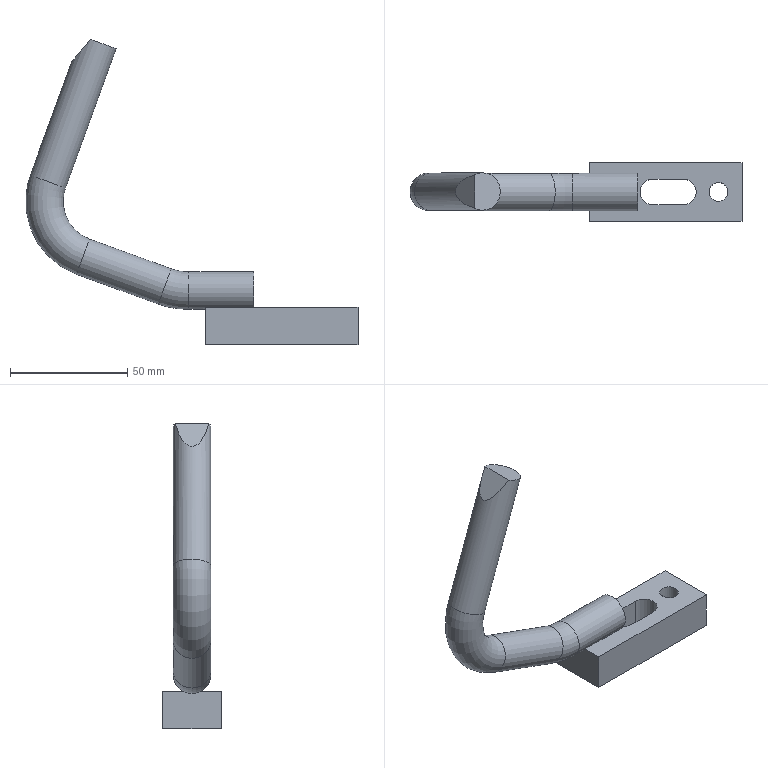Part | NX | features MAIN_BODY 2 | 1 solid | 19 faces | box 141.738 x 25 x 130.205 mm | volume 56808 mm3 | plane 10 | cylinder 6 | torus 2 | spline 1 | commonest cylinder face diameters 16 x3 11 x2 8 x1
STEP:
#1=CARTESIAN_POINT('',(970.,301.373,-139.));
#2=VERTEX_POINT('',#1);
#3=CARTESIAN_POINT('',(970.,293.627,-139.));
#4=VERTEX_POINT('',#3);
#5=CARTESIAN_POINT('',(970.,297.5,-132.));
#6=DIRECTION('',(1.,0.,0.));
#7=DIRECTION('',(0.,1.,0.));
#8=AXIS2_PLACEMENT_3D('',#5,#6,#7);
#9=CIRCLE('',#8,8.);
#10=EDGE_CURVE('',#2,#4,#9,.F.);
#11=ORIENTED_EDGE('',*,*,#10,.F.);
#12=CARTESIAN_POINT('',(970.,310.,-139.));
#13=VERTEX_POINT('',#12);
#14=CARTESIAN_POINT('',(970.,285.5,-139.));
#15=DIRECTION('',(0.,-1.,0.));
#16=VECTOR('',#15,1000.);
#17=LINE('',#14,#16);
#18=EDGE_CURVE('',#2,#13,#17,.F.);
#19=ORIENTED_EDGE('',*,*,#18,.T.);
#20=CARTESIAN_POINT('',(970.,310.,-155.));
#21=VERTEX_POINT('',#20);
#22=CARTESIAN_POINT('',(970.,310.,-135.));
#23=DIRECTION('',(0.,0.,1.));
#24=VECTOR('',#23,1000.);
#25=LINE('',#22,#24);
#26=EDGE_CURVE('',#21,#13,#25,.T.);
#27=ORIENTED_EDGE('',*,*,#26,.F.);
#28=CARTESIAN_POINT('',(970.,285.,-155.));
#29=VERTEX_POINT('',#28);
#30=CARTESIAN_POINT('',(970.,285.5,-155.));
#31=DIRECTION('',(0.,-1.,0.));
#32=VECTOR('',#31,1000.);
#33=LINE('',#30,#32);
#34=EDGE_CURVE('',#29,#21,#33,.F.);
#35=ORIENTED_EDGE('',*,*,#34,.F.);
#36=CARTESIAN_POINT('',(970.,285.,-139.));
#37=VERTEX_POINT('',#36);
#38=CARTESIAN_POINT('',(970.,285.,-135.));
#39=DIRECTION('',(0.,0.,-1.));
#40=VECTOR('',#39,1000.);
#41=LINE('',#38,#40);
#42=EDGE_CURVE('',#29,#37,#41,.F.);
#43=ORIENTED_EDGE('',*,*,#42,.T.);
#44=CARTESIAN_POINT('',(970.,285.5,-139.));
#45=DIRECTION('',(0.,-1.,0.));
#46=VECTOR('',#45,1000.);
#47=LINE('',#44,#46);
#48=EDGE_CURVE('',#37,#4,#47,.F.);
#49=ORIENTED_EDGE('',*,*,#48,.T.);
#50=EDGE_LOOP('',(#11,#19,#27,#35,#43,#49));
#51=FACE_BOUND('',#50,.T.);
#52=CARTESIAN_POINT('',(970.,285.5,-135.));
#53=DIRECTION('',(1.,0.,0.));
#54=DIRECTION('',(0.,1.,0.));
#55=AXIS2_PLACEMENT_3D('',#52,#53,#54);
#56=PLANE('',#55);
#57=ADVANCED_FACE('',(#51),#56,.F.);
#58=ORIENTED_EDGE('',*,*,#18,.F.);
#59=CARTESIAN_POINT('',(990.552,301.373,-139.));
#60=VERTEX_POINT('',#59);
#61=CARTESIAN_POINT('',(962.842,301.373,-139.));
#62=DIRECTION('',(1.,0.,0.));
#63=VECTOR('',#62,1000.);
#64=LINE('',#61,#63);
#65=EDGE_CURVE('',#2,#60,#64,.T.);
#66=ORIENTED_EDGE('',*,*,#65,.T.);
#67=CARTESIAN_POINT('',(990.552,293.627,-139.));
#68=VERTEX_POINT('',#67);
#69=CARTESIAN_POINT('',(990.552,285.5,-139.));
#70=DIRECTION('',(0.,-1.,0.));
#71=VECTOR('',#70,1000.);
#72=LINE('',#69,#71);
#73=EDGE_CURVE('',#60,#68,#72,.T.);
#74=ORIENTED_EDGE('',*,*,#73,.T.);
#75=CARTESIAN_POINT('',(962.842,293.627,-139.));
#76=DIRECTION('',(1.,0.,0.));
#77=VECTOR('',#76,1000.);
#78=LINE('',#75,#77);
#79=EDGE_CURVE('',#68,#4,#78,.F.);
#80=ORIENTED_EDGE('',*,*,#79,.T.);
#81=ORIENTED_EDGE('',*,*,#48,.F.);
#82=CARTESIAN_POINT('',(1035.,285.,-139.));
#83=VERTEX_POINT('',#82);
#84=CARTESIAN_POINT('',(900.,285.,-139.));
#85=DIRECTION('',(1.,0.,0.));
#86=VECTOR('',#85,1000.);
#87=LINE('',#84,#86);
#88=EDGE_CURVE('',#37,#83,#87,.T.);
#89=ORIENTED_EDGE('',*,*,#88,.T.);
#90=CARTESIAN_POINT('',(1035.,310.,-139.));
#91=VERTEX_POINT('',#90);
#92=CARTESIAN_POINT('',(1035.,285.5,-139.));
#93=DIRECTION('',(0.,1.,0.));
#94=VECTOR('',#93,1000.);
#95=LINE('',#92,#94);
#96=EDGE_CURVE('',#83,#91,#95,.T.);
#97=ORIENTED_EDGE('',*,*,#96,.T.);
#98=CARTESIAN_POINT('',(900.,310.,-139.));
#99=DIRECTION('',(-1.,0.,0.));
#100=VECTOR('',#99,1000.);
#101=LINE('',#98,#100);
#102=EDGE_CURVE('',#13,#91,#101,.F.);
#103=ORIENTED_EDGE('',*,*,#102,.F.);
#104=EDGE_LOOP('',(#58,#66,#74,#80,#81,#89,#97,#103));
#105=FACE_BOUND('',#104,.T.);
#106=CARTESIAN_POINT('',(1021.,297.5,-139.));
#107=VERTEX_POINT('',#106);
#108=CARTESIAN_POINT('',(1025.,297.5,-139.));
#109=DIRECTION('',(0.,0.,-1.));
#110=DIRECTION('',(-1.,0.,0.));
#111=AXIS2_PLACEMENT_3D('',#108,#109,#110);
#112=CIRCLE('',#111,4.);
#113=EDGE_CURVE('',#107,#107,#112,.F.);
#114=ORIENTED_EDGE('',*,*,#113,.F.);
#115=EDGE_LOOP('',(#114));
#116=FACE_BOUND('',#115,.T.);
#117=CARTESIAN_POINT('',(1010.,292.,-139.));
#118=VERTEX_POINT('',#117);
#119=CARTESIAN_POINT('',(1010.,303.,-139.));
#120=VERTEX_POINT('',#119);
#121=CARTESIAN_POINT('',(1010.,297.5,-139.));
#122=DIRECTION('',(0.,0.,-1.));
#123=DIRECTION('',(-1.,0.,0.));
#124=AXIS2_PLACEMENT_3D('',#121,#122,#123);
#125=CIRCLE('',#124,5.5);
#126=EDGE_CURVE('',#118,#120,#125,.F.);
#127=ORIENTED_EDGE('',*,*,#126,.F.);
#128=CARTESIAN_POINT('',(997.,292.,-139.));
#129=VERTEX_POINT('',#128);
#130=CARTESIAN_POINT('',(969.,292.,-139.));
#131=DIRECTION('',(-1.,0.,0.));
#132=VECTOR('',#131,1000.);
#133=LINE('',#130,#132);
#134=EDGE_CURVE('',#129,#118,#133,.F.);
#135=ORIENTED_EDGE('',*,*,#134,.F.);
#136=CARTESIAN_POINT('',(997.,303.,-139.));
#137=VERTEX_POINT('',#136);
#138=CARTESIAN_POINT('',(997.,297.5,-139.));
#139=DIRECTION('',(0.,0.,-1.));
#140=DIRECTION('',(-1.,0.,0.));
#141=AXIS2_PLACEMENT_3D('',#138,#139,#140);
#142=CIRCLE('',#141,5.5);
#143=EDGE_CURVE('',#137,#129,#142,.F.);
#144=ORIENTED_EDGE('',*,*,#143,.F.);
#145=CARTESIAN_POINT('',(969.,303.,-139.));
#146=DIRECTION('',(-1.,0.,0.));
#147=VECTOR('',#146,1000.);
#148=LINE('',#145,#147);
#149=EDGE_CURVE('',#120,#137,#148,.T.);
#150=ORIENTED_EDGE('',*,*,#149,.F.);
#151=EDGE_LOOP('',(#127,#135,#144,#150));
#152=FACE_BOUND('',#151,.T.);
#153=CARTESIAN_POINT('',(900.,285.5,-139.));
#154=DIRECTION('',(0.,0.,-1.));
#155=DIRECTION('',(-1.,0.,0.));
#156=AXIS2_PLACEMENT_3D('',#153,#154,#155);
#157=PLANE('',#156);
#158=ADVANCED_FACE('',(#105,#116,#152),#157,.F.);
#159=CARTESIAN_POINT('',(1035.,285.,-155.));
#160=VERTEX_POINT('',#159);
#161=CARTESIAN_POINT('',(1035.,285.,-135.));
#162=DIRECTION('',(0.,0.,1.));
#163=VECTOR('',#162,1000.);
#164=LINE('',#161,#163);
#165=EDGE_CURVE('',#160,#83,#164,.T.);
#166=ORIENTED_EDGE('',*,*,#165,.T.);
#167=ORIENTED_EDGE('',*,*,#88,.F.);
#168=ORIENTED_EDGE('',*,*,#42,.F.);
#169=CARTESIAN_POINT('',(900.,285.,-155.));
#170=DIRECTION('',(1.,0.,0.));
#171=VECTOR('',#170,1000.);
#172=LINE('',#169,#171);
#173=EDGE_CURVE('',#29,#160,#172,.T.);
#174=ORIENTED_EDGE('',*,*,#173,.T.);
#175=EDGE_LOOP('',(#166,#167,#168,#174));
#176=FACE_BOUND('',#175,.T.);
#177=CARTESIAN_POINT('',(900.,285.,-135.));
#178=DIRECTION('',(0.,-1.,0.));
#179=DIRECTION('',(1.,0.,0.));
#180=AXIS2_PLACEMENT_3D('',#177,#178,#179);
#181=PLANE('',#180);
#182=ADVANCED_FACE('',(#176),#181,.T.);
#183=ORIENTED_EDGE('',*,*,#26,.T.);
#184=ORIENTED_EDGE('',*,*,#102,.T.);
#185=CARTESIAN_POINT('',(1035.,310.,-155.));
#186=VERTEX_POINT('',#185);
#187=CARTESIAN_POINT('',(1035.,310.,-135.));
#188=DIRECTION('',(0.,0.,-1.));
#189=VECTOR('',#188,1000.);
#190=LINE('',#187,#189);
#191=EDGE_CURVE('',#186,#91,#190,.F.);
#192=ORIENTED_EDGE('',*,*,#191,.F.);
#193=CARTESIAN_POINT('',(900.,310.,-155.));
#194=DIRECTION('',(-1.,0.,0.));
#195=VECTOR('',#194,1000.);
#196=LINE('',#193,#195);
#197=EDGE_CURVE('',#21,#186,#196,.F.);
#198=ORIENTED_EDGE('',*,*,#197,.F.);
#199=EDGE_LOOP('',(#183,#184,#192,#198));
#200=FACE_BOUND('',#199,.T.);
#201=CARTESIAN_POINT('',(900.,310.,-135.));
#202=DIRECTION('',(0.,-1.,0.));
#203=DIRECTION('',(1.,0.,0.));
#204=AXIS2_PLACEMENT_3D('',#201,#202,#203);
#205=PLANE('',#204);
#206=ADVANCED_FACE('',(#200),#205,.F.);
#207=CARTESIAN_POINT('',(1035.,285.5,-155.));
#208=DIRECTION('',(0.,1.,0.));
#209=VECTOR('',#208,1000.);
#210=LINE('',#207,#209);
#211=EDGE_CURVE('',#160,#186,#210,.T.);
#212=ORIENTED_EDGE('',*,*,#211,.T.);
#213=ORIENTED_EDGE('',*,*,#191,.T.);
#214=ORIENTED_EDGE('',*,*,#96,.F.);
#215=ORIENTED_EDGE('',*,*,#165,.F.);
#216=EDGE_LOOP('',(#212,#213,#214,#215));
#217=FACE_BOUND('',#216,.T.);
#218=CARTESIAN_POINT('',(1035.,285.5,-135.));
#219=DIRECTION('',(1.,0.,0.));
#220=DIRECTION('',(0.,1.,0.));
#221=AXIS2_PLACEMENT_3D('',#218,#219,#220);
#222=PLANE('',#221);
#223=ADVANCED_FACE('',(#217),#222,.T.);
#224=CARTESIAN_POINT('',(1021.03,297.987,-155.));
#225=VERTEX_POINT('',#224);
#226=CARTESIAN_POINT('',(1025.,297.5,-155.));
#227=DIRECTION('',(0.,0.,1.));
#228=DIRECTION('',(-0.9925,0.1219,0.));
#229=AXIS2_PLACEMENT_3D('',#226,#227,#228);
#230=CIRCLE('',#229,4.);
#231=EDGE_CURVE('',#225,#225,#230,.T.);
#232=ORIENTED_EDGE('',*,*,#231,.T.);
#233=EDGE_LOOP('',(#232));
#234=FACE_BOUND('',#233,.T.);
#235=CARTESIAN_POINT('',(1010.,303.,-155.));
#236=VERTEX_POINT('',#235);
#237=CARTESIAN_POINT('',(997.,303.,-155.));
#238=VERTEX_POINT('',#237);
#239=CARTESIAN_POINT('',(969.,303.,-155.));
#240=DIRECTION('',(-1.,0.,0.));
#241=VECTOR('',#240,1000.);
#242=LINE('',#239,#241);
#243=EDGE_CURVE('',#236,#238,#242,.T.);
#244=ORIENTED_EDGE('',*,*,#243,.T.);
#245=CARTESIAN_POINT('',(997.,292.,-155.));
#246=VERTEX_POINT('',#245);
#247=CARTESIAN_POINT('',(997.,297.5,-155.));
#248=DIRECTION('',(0.,0.,-1.));
#249=DIRECTION('',(-0.9925,0.1219,0.));
#250=AXIS2_PLACEMENT_3D('',#247,#248,#249);
#251=CIRCLE('',#250,5.5);
#252=EDGE_CURVE('',#238,#246,#251,.F.);
#253=ORIENTED_EDGE('',*,*,#252,.T.);
#254=CARTESIAN_POINT('',(1010.,292.,-155.));
#255=VERTEX_POINT('',#254);
#256=CARTESIAN_POINT('',(969.,292.,-155.));
#257=DIRECTION('',(-1.,0.,0.));
#258=VECTOR('',#257,1000.);
#259=LINE('',#256,#258);
#260=EDGE_CURVE('',#246,#255,#259,.F.);
#261=ORIENTED_EDGE('',*,*,#260,.T.);
#262=CARTESIAN_POINT('',(1010.,297.5,-155.));
#263=DIRECTION('',(0.,0.,-1.));
#264=DIRECTION('',(-0.9925,0.1219,0.));
#265=AXIS2_PLACEMENT_3D('',#262,#263,#264);
#266=CIRCLE('',#265,5.5);
#267=EDGE_CURVE('',#255,#236,#266,.F.);
#268=ORIENTED_EDGE('',*,*,#267,.T.);
#269=EDGE_LOOP('',(#244,#253,#261,#268));
#270=FACE_BOUND('',#269,.T.);
#271=ORIENTED_EDGE('',*,*,#197,.T.);
#272=ORIENTED_EDGE('',*,*,#211,.F.);
#273=ORIENTED_EDGE('',*,*,#173,.F.);
#274=ORIENTED_EDGE('',*,*,#34,.T.);
#275=EDGE_LOOP('',(#271,#272,#273,#274));
#276=FACE_BOUND('',#275,.T.);
#277=CARTESIAN_POINT('',(900.,285.5,-155.));
#278=DIRECTION('',(0.,0.,-1.));
#279=DIRECTION('',(-1.,0.,0.));
#280=AXIS2_PLACEMENT_3D('',#277,#278,#279);
#281=PLANE('',#280);
#282=ADVANCED_FACE('',(#234,#270,#276),#281,.T.);
#283=ORIENTED_EDGE('',*,*,#143,.T.);
#284=CARTESIAN_POINT('',(997.,292.,-119.));
#285=DIRECTION('',(0.,0.,-1.));
#286=VECTOR('',#285,1000.);
#287=LINE('',#284,#286);
#288=EDGE_CURVE('',#129,#246,#287,.T.);
#289=ORIENTED_EDGE('',*,*,#288,.T.);
#290=ORIENTED_EDGE('',*,*,#252,.F.);
#291=CARTESIAN_POINT('',(997.,303.,-119.));
#292=DIRECTION('',(0.,0.,-1.));
#293=VECTOR('',#292,1000.);
#294=LINE('',#291,#293);
#295=EDGE_CURVE('',#137,#238,#294,.T.);
#296=ORIENTED_EDGE('',*,*,#295,.F.);
#297=EDGE_LOOP('',(#283,#289,#290,#296));
#298=FACE_BOUND('',#297,.T.);
#299=CARTESIAN_POINT('',(997.,297.5,-119.));
#300=DIRECTION('',(0.,0.,-1.));
#301=DIRECTION('',(-1.,0.,0.));
#302=AXIS2_PLACEMENT_3D('',#299,#300,#301);
#303=CYLINDRICAL_SURFACE('',#302,5.5);
#304=ADVANCED_FACE('',(#298),#303,.F.);
#305=ORIENTED_EDGE('',*,*,#126,.T.);
#306=CARTESIAN_POINT('',(1010.,303.,-119.));
#307=DIRECTION('',(0.,0.,-1.));
#308=VECTOR('',#307,1000.);
#309=LINE('',#306,#308);
#310=EDGE_CURVE('',#120,#236,#309,.T.);
#311=ORIENTED_EDGE('',*,*,#310,.T.);
#312=ORIENTED_EDGE('',*,*,#267,.F.);
#313=CARTESIAN_POINT('',(1010.,292.,-119.));
#314=DIRECTION('',(0.,0.,-1.));
#315=VECTOR('',#314,1000.);
#316=LINE('',#313,#315);
#317=EDGE_CURVE('',#118,#255,#316,.T.);
#318=ORIENTED_EDGE('',*,*,#317,.F.);
#319=EDGE_LOOP('',(#305,#311,#312,#318));
#320=FACE_BOUND('',#319,.T.);
#321=CARTESIAN_POINT('',(1010.,297.5,-119.));
#322=DIRECTION('',(0.,0.,-1.));
#323=DIRECTION('',(-1.,0.,0.));
#324=AXIS2_PLACEMENT_3D('',#321,#322,#323);
#325=CYLINDRICAL_SURFACE('',#324,5.5);
#326=ADVANCED_FACE('',(#320),#325,.F.);
#327=ORIENTED_EDGE('',*,*,#310,.F.);
#328=ORIENTED_EDGE('',*,*,#149,.T.);
#329=ORIENTED_EDGE('',*,*,#295,.T.);
#330=ORIENTED_EDGE('',*,*,#243,.F.);
#331=EDGE_LOOP('',(#327,#328,#329,#330));
#332=FACE_BOUND('',#331,.T.);
#333=CARTESIAN_POINT('',(969.,303.,-119.));
#334=DIRECTION('',(0.,1.,0.));
#335=DIRECTION('',(-1.,0.,0.));
#336=AXIS2_PLACEMENT_3D('',#333,#334,#335);
#337=PLANE('',#336);
#338=ADVANCED_FACE('',(#332),#337,.F.);
#339=ORIENTED_EDGE('',*,*,#288,.F.);
#340=ORIENTED_EDGE('',*,*,#134,.T.);
#341=ORIENTED_EDGE('',*,*,#317,.T.);
#342=ORIENTED_EDGE('',*,*,#260,.F.);
#343=EDGE_LOOP('',(#339,#340,#341,#342));
#344=FACE_BOUND('',#343,.T.);
#345=CARTESIAN_POINT('',(969.,292.,-119.));
#346=DIRECTION('',(0.,1.,0.));
#347=DIRECTION('',(-1.,0.,0.));
#348=AXIS2_PLACEMENT_3D('',#345,#346,#347);
#349=PLANE('',#348);
#350=ADVANCED_FACE('',(#344),#349,.T.);
#351=ORIENTED_EDGE('',*,*,#231,.F.);
#352=EDGE_LOOP('',(#351));
#353=FACE_BOUND('',#352,.T.);
#354=ORIENTED_EDGE('',*,*,#113,.T.);
#355=EDGE_LOOP('',(#354));
#356=FACE_BOUND('',#355,.T.);
#357=CARTESIAN_POINT('',(1025.,297.5,-139.));
#358=DIRECTION('',(0.,0.,-1.));
#359=DIRECTION('',(-0.9925,0.1219,0.));
#360=AXIS2_PLACEMENT_3D('',#357,#358,#359);
#361=CYLINDRICAL_SURFACE('',#360,4.);
#362=ADVANCED_FACE('',(#353,#356),#361,.F.);
#363=CARTESIAN_POINT('',(962.842,297.5,-140.));
#364=VERTEX_POINT('',#363);
#365=CARTESIAN_POINT('',(962.842,297.5,-132.));
#366=DIRECTION('',(1.,0.,0.));
#367=DIRECTION('',(0.,0.,-1.));
#368=AXIS2_PLACEMENT_3D('',#365,#366,#367);
#369=CIRCLE('',#368,8.);
#370=EDGE_CURVE('',#364,#364,#369,.T.);
#371=ORIENTED_EDGE('',*,*,#370,.T.);
#372=EDGE_LOOP('',(#371));
#373=FACE_BOUND('',#372,.T.);
#374=ORIENTED_EDGE('',*,*,#65,.F.);
#375=ORIENTED_EDGE('',*,*,#10,.T.);
#376=ORIENTED_EDGE('',*,*,#79,.F.);
#377=CARTESIAN_POINT('',(990.552,297.5,-132.));
#378=DIRECTION('',(1.,0.,0.));
#379=DIRECTION('',(0.,0.,-1.));
#380=AXIS2_PLACEMENT_3D('',#377,#378,#379);
#381=CIRCLE('',#380,8.);
#382=EDGE_CURVE('',#60,#68,#381,.T.);
#383=ORIENTED_EDGE('',*,*,#382,.F.);
#384=EDGE_LOOP('',(#374,#375,#376,#383));
#385=FACE_BOUND('',#384,.T.);
#386=CARTESIAN_POINT('',(962.842,297.5,-132.));
#387=DIRECTION('',(1.,0.,0.));
#388=DIRECTION('',(0.,0.,-1.));
#389=AXIS2_PLACEMENT_3D('',#386,#387,#388);
#390=CYLINDRICAL_SURFACE('',#389,8.);
#391=ADVANCED_FACE('',(#373,#385),#390,.T.);
#392=ORIENTED_EDGE('',*,*,#73,.F.);
#393=ORIENTED_EDGE('',*,*,#382,.T.);
#394=EDGE_LOOP('',(#392,#393));
#395=FACE_BOUND('',#394,.T.);
#396=CARTESIAN_POINT('',(990.552,297.5,-132.));
#397=DIRECTION('',(1.,0.,0.));
#398=DIRECTION('',(0.,0.,-1.));
#399=AXIS2_PLACEMENT_3D('',#396,#397,#398);
#400=PLANE('',#399);
#401=ADVANCED_FACE('',(#395),#400,.T.);
#402=CARTESIAN_POINT('',(895.252,297.5,-82.72));
#403=VERTEX_POINT('',#402);
#404=CARTESIAN_POINT('',(902.769,297.5,-85.456));
#405=DIRECTION('',(-0.342,0.,-0.9397));
#406=DIRECTION('',(-0.9397,0.,0.342));
#407=AXIS2_PLACEMENT_3D('',#404,#405,#406);
#408=CIRCLE('',#407,8.);
#409=EDGE_CURVE('',#403,#403,#408,.T.);
#410=ORIENTED_EDGE('',*,*,#409,.F.);
#411=EDGE_LOOP('',(#410));
#412=FACE_BOUND('',#411,.T.);
#413=CARTESIAN_POINT('',(920.975,304.624,-24.795));
#414=VERTEX_POINT('',#413);
#415=CARTESIAN_POINT('',(920.975,290.376,-24.795));
#416=VERTEX_POINT('',#415);
#417=CARTESIAN_POINT('',(924.395,297.5,-26.04));
#418=DIRECTION('',(-0.342,0.,-0.9397));
#419=DIRECTION('',(-0.9397,0.,0.342));
#420=AXIS2_PLACEMENT_3D('',#417,#418,#419);
#421=CIRCLE('',#420,8.);
#422=EDGE_CURVE('',#414,#416,#421,.T.);
#423=ORIENTED_EDGE('',*,*,#422,.T.);
#424=CARTESIAN_POINT('',(920.975,290.376,-24.795));
#425=CARTESIAN_POINT('',(920.16,290.597,-25.766));
#426=CARTESIAN_POINT('',(918.549,291.134,-27.686));
#427=CARTESIAN_POINT('',(916.586,292.114,-30.026));
#428=CARTESIAN_POINT('',(915.08,293.202,-31.821));
#429=CARTESIAN_POINT('',(914.033,294.226,-33.068));
#430=CARTESIAN_POINT('',(913.117,295.557,-34.16));
#431=CARTESIAN_POINT('',(912.618,297.47,-34.754));
#432=CARTESIAN_POINT('',(913.094,299.401,-34.187));
#433=CARTESIAN_POINT('',(914.014,300.754,-33.091));
#434=CARTESIAN_POINT('',(915.069,301.79,-31.834));
#435=CARTESIAN_POINT('',(916.584,302.886,-30.027));
#436=CARTESIAN_POINT('',(918.541,303.862,-27.696));
#437=CARTESIAN_POINT('',(920.158,304.402,-25.769));
#438=CARTESIAN_POINT('',(920.975,304.624,-24.795));
#439=B_SPLINE_CURVE_WITH_KNOTS('',3,(#424,#425,#426,#427,#428,#429,#430,#431,#432,#433,#434,#435,#436,#437,#438),.UNSPECIFIED.,.F.,.F.,(4,1,1,1,1,1,1,1,1,1,1,1,4),(0.,0.00384,0.00768,0.0096,0.01152,0.01344,0.01536,0.01728,0.0192,0.02112,0.02304,0.02688,0.03072),.UNSPECIFIED.);
#440=EDGE_CURVE('',#416,#414,#439,.T.);
#441=ORIENTED_EDGE('',*,*,#440,.T.);
#442=EDGE_LOOP('',(#423,#441));
#443=FACE_BOUND('',#442,.T.);
#444=CARTESIAN_POINT('',(902.769,297.5,-85.456));
#445=DIRECTION('',(0.342,0.,0.9397));
#446=DIRECTION('',(0.9397,0.,-0.342));
#447=AXIS2_PLACEMENT_3D('',#444,#445,#446);
#448=CYLINDRICAL_SURFACE('',#447,8.);
#449=ADVANCED_FACE('',(#412,#443),#448,.T.);
#450=CARTESIAN_POINT('',(914.975,297.5,-125.017));
#451=VERTEX_POINT('',#450);
#452=CARTESIAN_POINT('',(917.711,297.5,-117.499));
#453=DIRECTION('',(0.9397,0.,-0.342));
#454=DIRECTION('',(-0.342,0.,-0.9397));
#455=AXIS2_PLACEMENT_3D('',#452,#453,#454);
#456=CIRCLE('',#455,8.);
#457=EDGE_CURVE('',#451,#451,#456,.T.);
#458=ORIENTED_EDGE('',*,*,#457,.F.);
#459=EDGE_LOOP('',(#458));
#460=FACE_BOUND('',#459,.T.);
#461=ORIENTED_EDGE('',*,*,#409,.T.);
#462=EDGE_LOOP('',(#461));
#463=FACE_BOUND('',#462,.T.);
#464=CARTESIAN_POINT('',(926.262,297.5,-94.007));
#465=DIRECTION('',(0.,1.,0.));
#466=DIRECTION('',(0.,0.,1.));
#467=AXIS2_PLACEMENT_3D('',#464,#465,#466);
#468=TOROIDAL_SURFACE('',#467,25.,8.);
#469=ADVANCED_FACE('',(#460,#463),#468,.T.);
#470=CARTESIAN_POINT('',(949.845,297.5,-137.708));
#471=VERTEX_POINT('',#470);
#472=CARTESIAN_POINT('',(952.581,297.5,-130.191));
#473=DIRECTION('',(0.9397,0.,-0.342));
#474=DIRECTION('',(-0.342,0.,-0.9397));
#475=AXIS2_PLACEMENT_3D('',#472,#473,#474);
#476=CIRCLE('',#475,8.);
#477=EDGE_CURVE('',#471,#471,#476,.T.);
#478=ORIENTED_EDGE('',*,*,#477,.F.);
#479=EDGE_LOOP('',(#478));
#480=FACE_BOUND('',#479,.T.);
#481=ORIENTED_EDGE('',*,*,#457,.T.);
#482=EDGE_LOOP('',(#481));
#483=FACE_BOUND('',#482,.T.);
#484=CARTESIAN_POINT('',(952.581,297.5,-130.191));
#485=DIRECTION('',(-0.9397,0.,0.342));
#486=DIRECTION('',(0.342,0.,0.9397));
#487=AXIS2_PLACEMENT_3D('',#484,#485,#486);
#488=CYLINDRICAL_SURFACE('',#487,8.);
#489=ADVANCED_FACE('',(#480,#483),#488,.T.);
#490=ORIENTED_EDGE('',*,*,#370,.F.);
#491=EDGE_LOOP('',(#490));
#492=FACE_BOUND('',#491,.T.);
#493=ORIENTED_EDGE('',*,*,#477,.T.);
#494=EDGE_LOOP('',(#493));
#495=FACE_BOUND('',#494,.T.);
#496=CARTESIAN_POINT('',(962.842,297.5,-102.));
#497=DIRECTION('',(0.,1.,0.));
#498=DIRECTION('',(0.,0.,1.));
#499=AXIS2_PLACEMENT_3D('',#496,#497,#498);
#500=TOROIDAL_SURFACE('',#499,30.,8.);
#501=ADVANCED_FACE('',(#492,#495),#500,.T.);
#502=ORIENTED_EDGE('',*,*,#422,.F.);
#503=CARTESIAN_POINT('',(920.975,290.376,-24.795));
#504=CARTESIAN_POINT('',(920.975,295.125,-24.795));
#505=CARTESIAN_POINT('',(920.975,299.875,-24.795));
#506=CARTESIAN_POINT('',(920.975,304.624,-24.795));
#507=B_SPLINE_CURVE_WITH_KNOTS('',3,(#503,#504,#505,#506),.UNSPECIFIED.,.F.,.F.,(4,4),(0.008121,0.02237),.UNSPECIFIED.);
#508=EDGE_CURVE('',#414,#416,#507,.F.);
#509=ORIENTED_EDGE('',*,*,#508,.T.);
#510=EDGE_LOOP('',(#502,#509));
#511=FACE_BOUND('',#510,.T.);
#512=CARTESIAN_POINT('',(924.395,297.5,-26.04));
#513=DIRECTION('',(-0.342,0.,-0.9397));
#514=DIRECTION('',(-0.9397,0.,0.342));
#515=AXIS2_PLACEMENT_3D('',#512,#513,#514);
#516=PLANE('',#515);
#517=ADVANCED_FACE('',(#511),#516,.F.);
#518=ORIENTED_EDGE('',*,*,#508,.F.);
#519=ORIENTED_EDGE('',*,*,#440,.F.);
#520=EDGE_LOOP('',(#518,#519));
#521=FACE_BOUND('',#520,.T.);
#522=CARTESIAN_POINT('',(920.975,290.29,-24.795));
#523=CARTESIAN_POINT('',(920.975,304.71,-24.795));
#524=CARTESIAN_POINT('',(912.719,290.29,-34.634));
#525=CARTESIAN_POINT('',(912.719,304.71,-34.634));
#526=B_SPLINE_SURFACE_WITH_KNOTS('',1,1,((#522,#523),(#524,#525)),.PLANE_SURF.,.F.,.F.,.F.,(2,2),(2,2),(0.4841,0.666),(0.3516,0.6484),.PIECEWISE_BEZIER_KNOTS.);
#527=ADVANCED_FACE('',(#521),#526,.F.);
#528=CLOSED_SHELL('',(#57,#158,#182,#206,#223,#282,#304,#326,#338,#350,#362,#391,#401,#449,#469,#489,#501,#517,#527));
#529=MANIFOLD_SOLID_BREP('',#528);
#530=(LENGTH_UNIT()NAMED_UNIT(*)SI_UNIT(.MILLI.,.METRE.));
#531=UNCERTAINTY_MEASURE_WITH_UNIT(LENGTH_MEASURE(0.0508),#530,'','');
#532=(NAMED_UNIT(*)PLANE_ANGLE_UNIT()SI_UNIT($,.RADIAN.));
#533=(NAMED_UNIT(*)SI_UNIT($,.STERADIAN.)SOLID_ANGLE_UNIT());
#534=(GEOMETRIC_REPRESENTATION_CONTEXT(3)GLOBAL_UNCERTAINTY_ASSIGNED_CONTEXT((#531))GLOBAL_UNIT_ASSIGNED_CONTEXT((#530,#532,#533))REPRESENTATION_CONTEXT('',''));
#535=ADVANCED_BREP_SHAPE_REPRESENTATION('',(#529),#534);